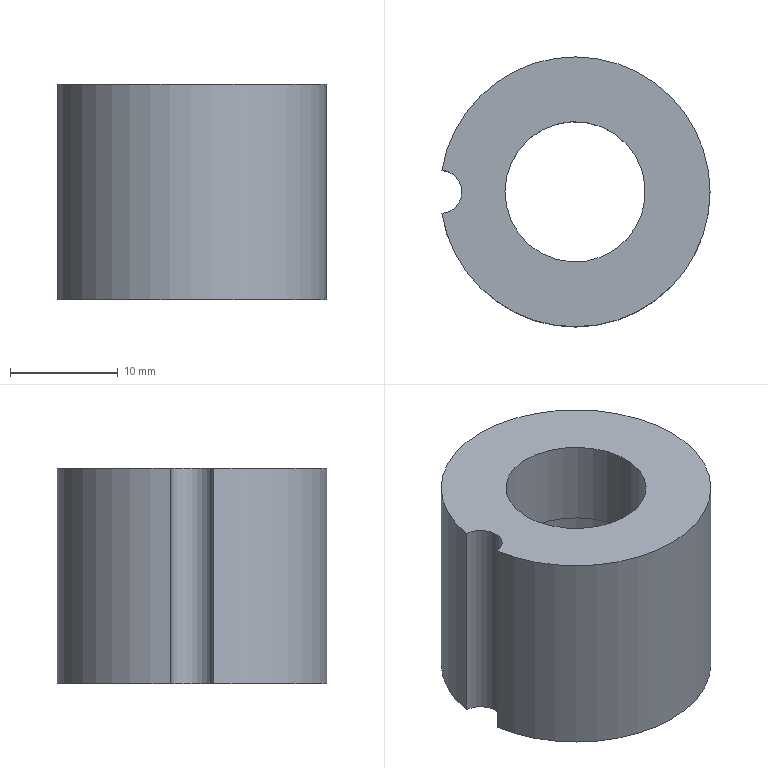Part | NX | features solid 2 | 1 solid | 7 faces | box 24.84 x 25 x 20 mm | volume 6037 mm3 | cylinder 4 | plane 3 | commonest cylinder face diameters 4 x1 13 x1 16.6 x1 25 x1
STEP:
#1=CARTESIAN_POINT('',(1506.718,315.94,3.4));
#2=VERTEX_POINT('',#1);
#3=CARTESIAN_POINT('',(1506.718,315.94,23.4));
#4=VERTEX_POINT('',#3);
#5=CARTESIAN_POINT('',(1506.718,315.94,10.9));
#6=DIRECTION('',(0.,0.,1.));
#7=VECTOR('',#6,1000.);
#8=LINE('',#5,#7);
#9=EDGE_CURVE('',#2,#4,#8,.T.);
#10=ORIENTED_EDGE('',*,*,#9,.T.);
#11=CARTESIAN_POINT('',(1506.718,311.953,23.4));
#12=VERTEX_POINT('',#11);
#13=CARTESIAN_POINT('',(1519.058,313.947,23.4));
#14=DIRECTION('',(0.,0.,-1.));
#15=DIRECTION('',(-1.,0.,0.));
#16=AXIS2_PLACEMENT_3D('',#13,#14,#15);
#17=CIRCLE('',#16,12.5);
#18=EDGE_CURVE('',#4,#12,#17,.T.);
#19=ORIENTED_EDGE('',*,*,#18,.T.);
#20=CARTESIAN_POINT('',(1506.718,311.953,3.4));
#21=VERTEX_POINT('',#20);
#22=CARTESIAN_POINT('',(1506.718,311.953,10.9));
#23=DIRECTION('',(0.,0.,1.));
#24=VECTOR('',#23,1000.);
#25=LINE('',#22,#24);
#26=EDGE_CURVE('',#12,#21,#25,.F.);
#27=ORIENTED_EDGE('',*,*,#26,.T.);
#28=CARTESIAN_POINT('',(1519.058,313.947,3.4));
#29=DIRECTION('',(0.,0.,1.));
#30=DIRECTION('',(1.,0.,0.));
#31=AXIS2_PLACEMENT_3D('',#28,#29,#30);
#32=CIRCLE('',#31,12.5);
#33=EDGE_CURVE('',#2,#21,#32,.F.);
#34=ORIENTED_EDGE('',*,*,#33,.F.);
#35=EDGE_LOOP('',(#10,#19,#27,#34));
#36=FACE_BOUND('',#35,.T.);
#37=CARTESIAN_POINT('',(1519.058,313.947,-1.6));
#38=DIRECTION('',(0.,0.,1.));
#39=DIRECTION('',(-1.,0.,0.));
#40=AXIS2_PLACEMENT_3D('',#37,#38,#39);
#41=CYLINDRICAL_SURFACE('',#40,12.5);
#42=ADVANCED_FACE('',(#36),#41,.T.);
#43=CARTESIAN_POINT('',(1527.358,313.947,3.4));
#44=VERTEX_POINT('',#43);
#45=CARTESIAN_POINT('',(1519.058,313.947,3.4));
#46=DIRECTION('',(0.,0.,1.));
#47=DIRECTION('',(1.,0.,0.));
#48=AXIS2_PLACEMENT_3D('',#45,#46,#47);
#49=CIRCLE('',#48,8.3);
#50=EDGE_CURVE('',#44,#44,#49,.F.);
#51=ORIENTED_EDGE('',*,*,#50,.F.);
#52=EDGE_LOOP('',(#51));
#53=FACE_BOUND('',#52,.T.);
#54=ORIENTED_EDGE('',*,*,#33,.T.);
#55=CARTESIAN_POINT('',(1506.558,313.947,3.4));
#56=DIRECTION('',(0.,0.,1.));
#57=DIRECTION('',(1.,0.,0.));
#58=AXIS2_PLACEMENT_3D('',#55,#56,#57);
#59=CIRCLE('',#58,2.);
#60=EDGE_CURVE('',#2,#21,#59,.F.);
#61=ORIENTED_EDGE('',*,*,#60,.F.);
#62=EDGE_LOOP('',(#54,#61));
#63=FACE_BOUND('',#62,.T.);
#64=CARTESIAN_POINT('',(1519.058,313.947,3.4));
#65=DIRECTION('',(0.,0.,1.));
#66=DIRECTION('',(-1.,0.,0.));
#67=AXIS2_PLACEMENT_3D('',#64,#65,#66);
#68=PLANE('',#67);
#69=ADVANCED_FACE('',(#53,#63),#68,.F.);
#70=CARTESIAN_POINT('',(1512.558,313.947,23.4));
#71=VERTEX_POINT('',#70);
#72=CARTESIAN_POINT('',(1519.058,313.947,23.4));
#73=DIRECTION('',(0.,0.,-1.));
#74=DIRECTION('',(-1.,0.,0.));
#75=AXIS2_PLACEMENT_3D('',#72,#73,#74);
#76=CIRCLE('',#75,6.5);
#77=EDGE_CURVE('',#71,#71,#76,.T.);
#78=ORIENTED_EDGE('',*,*,#77,.T.);
#79=EDGE_LOOP('',(#78));
#80=FACE_BOUND('',#79,.T.);
#81=CARTESIAN_POINT('',(1506.558,313.947,23.4));
#82=DIRECTION('',(0.,0.,-1.));
#83=DIRECTION('',(-1.,0.,0.));
#84=AXIS2_PLACEMENT_3D('',#81,#82,#83);
#85=CIRCLE('',#84,2.);
#86=EDGE_CURVE('',#4,#12,#85,.T.);
#87=ORIENTED_EDGE('',*,*,#86,.T.);
#88=ORIENTED_EDGE('',*,*,#18,.F.);
#89=EDGE_LOOP('',(#87,#88));
#90=FACE_BOUND('',#89,.T.);
#91=CARTESIAN_POINT('',(1519.058,313.947,23.4));
#92=DIRECTION('',(0.,0.,1.));
#93=DIRECTION('',(-1.,0.,0.));
#94=AXIS2_PLACEMENT_3D('',#91,#92,#93);
#95=PLANE('',#94);
#96=ADVANCED_FACE('',(#80,#90),#95,.T.);
#97=ORIENTED_EDGE('',*,*,#50,.T.);
#98=EDGE_LOOP('',(#97));
#99=FACE_BOUND('',#98,.T.);
#100=CARTESIAN_POINT('',(1510.758,313.947,15.4));
#101=VERTEX_POINT('',#100);
#102=CARTESIAN_POINT('',(1519.058,313.947,15.4));
#103=DIRECTION('',(0.,0.,-1.));
#104=DIRECTION('',(-1.,0.,0.));
#105=AXIS2_PLACEMENT_3D('',#102,#103,#104);
#106=CIRCLE('',#105,8.3);
#107=EDGE_CURVE('',#101,#101,#106,.T.);
#108=ORIENTED_EDGE('',*,*,#107,.F.);
#109=EDGE_LOOP('',(#108));
#110=FACE_BOUND('',#109,.T.);
#111=CARTESIAN_POINT('',(1519.058,313.947,-1.6));
#112=DIRECTION('',(0.,0.,1.));
#113=DIRECTION('',(-1.,0.,0.));
#114=AXIS2_PLACEMENT_3D('',#111,#112,#113);
#115=CYLINDRICAL_SURFACE('',#114,8.3);
#116=ADVANCED_FACE('',(#99,#110),#115,.F.);
#117=CARTESIAN_POINT('',(1512.558,313.947,15.4));
#118=VERTEX_POINT('',#117);
#119=CARTESIAN_POINT('',(1519.058,313.947,15.4));
#120=DIRECTION('',(0.,0.,-1.));
#121=DIRECTION('',(-1.,0.,0.));
#122=AXIS2_PLACEMENT_3D('',#119,#120,#121);
#123=CIRCLE('',#122,6.5);
#124=EDGE_CURVE('',#118,#118,#123,.T.);
#125=ORIENTED_EDGE('',*,*,#124,.F.);
#126=EDGE_LOOP('',(#125));
#127=FACE_BOUND('',#126,.T.);
#128=ORIENTED_EDGE('',*,*,#107,.T.);
#129=EDGE_LOOP('',(#128));
#130=FACE_BOUND('',#129,.T.);
#131=CARTESIAN_POINT('',(1519.058,313.947,15.4));
#132=DIRECTION('',(0.,0.,1.));
#133=DIRECTION('',(-1.,0.,0.));
#134=AXIS2_PLACEMENT_3D('',#131,#132,#133);
#135=PLANE('',#134);
#136=ADVANCED_FACE('',(#127,#130),#135,.F.);
#137=ORIENTED_EDGE('',*,*,#9,.F.);
#138=ORIENTED_EDGE('',*,*,#60,.T.);
#139=ORIENTED_EDGE('',*,*,#26,.F.);
#140=ORIENTED_EDGE('',*,*,#86,.F.);
#141=EDGE_LOOP('',(#137,#138,#139,#140));
#142=FACE_BOUND('',#141,.T.);
#143=CARTESIAN_POINT('',(1506.558,313.947,-1.6));
#144=DIRECTION('',(0.,0.,1.));
#145=DIRECTION('',(-1.,0.,0.));
#146=AXIS2_PLACEMENT_3D('',#143,#144,#145);
#147=CYLINDRICAL_SURFACE('',#146,2.);
#148=ADVANCED_FACE('',(#142),#147,.F.);
#149=ORIENTED_EDGE('',*,*,#77,.F.);
#150=EDGE_LOOP('',(#149));
#151=FACE_BOUND('',#150,.T.);
#152=ORIENTED_EDGE('',*,*,#124,.T.);
#153=EDGE_LOOP('',(#152));
#154=FACE_BOUND('',#153,.T.);
#155=CARTESIAN_POINT('',(1519.058,313.947,-1.6));
#156=DIRECTION('',(0.,0.,1.));
#157=DIRECTION('',(-1.,0.,0.));
#158=AXIS2_PLACEMENT_3D('',#155,#156,#157);
#159=CYLINDRICAL_SURFACE('',#158,6.5);
#160=ADVANCED_FACE('',(#151,#154),#159,.F.);
#161=CLOSED_SHELL('',(#42,#69,#96,#116,#136,#148,#160));
#162=MANIFOLD_SOLID_BREP('',#161);
#163=(LENGTH_UNIT()NAMED_UNIT(*)SI_UNIT(.MILLI.,.METRE.));
#164=UNCERTAINTY_MEASURE_WITH_UNIT(LENGTH_MEASURE(0.00001),#163,'','');
#165=(NAMED_UNIT(*)PLANE_ANGLE_UNIT()SI_UNIT($,.RADIAN.));
#166=(NAMED_UNIT(*)SI_UNIT($,.STERADIAN.)SOLID_ANGLE_UNIT());
#167=(GEOMETRIC_REPRESENTATION_CONTEXT(3)GLOBAL_UNCERTAINTY_ASSIGNED_CONTEXT((#164))GLOBAL_UNIT_ASSIGNED_CONTEXT((#163,#165,#166))REPRESENTATION_CONTEXT('',''));
#168=ADVANCED_BREP_SHAPE_REPRESENTATION('',(#162),#167);